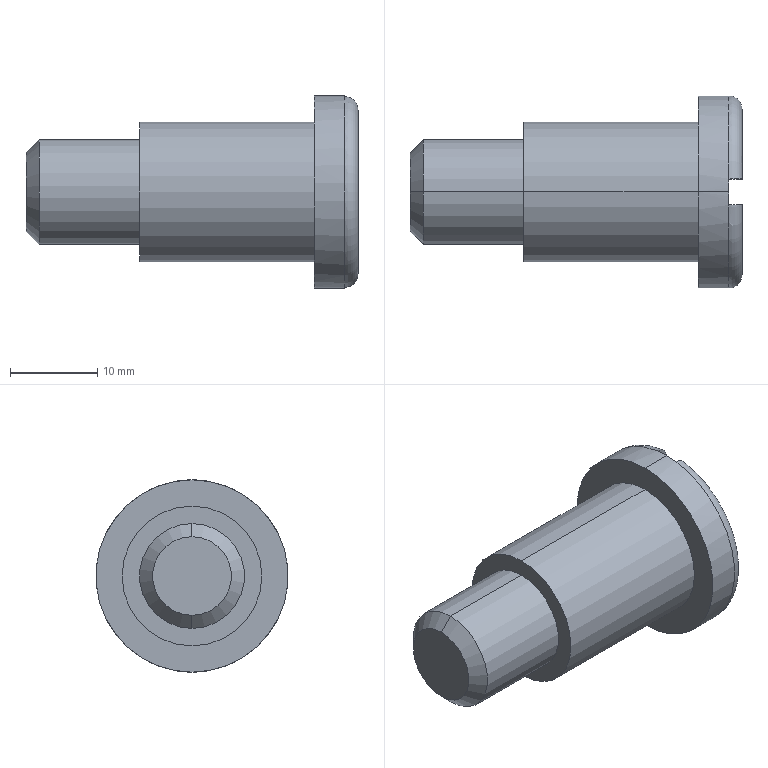Part | SolidWorks | features Chamfer 1, Cut 1, Fillet 1, Revolution 1 | 1 solid | 18 faces | box 38 x 22 x 22 mm | volume 7225 mm3 | plane 8 | cylinder 6 | cone 2 | torus 2 | commonest cylinder face diameters 12 x2 16 x2 22 x2
STEP:
#1=CARTESIAN_POINT('',(-19.,0.,4.5));
#2=VERTEX_POINT('',#1);
#3=CARTESIAN_POINT('',(-19.,0.,-4.5));
#4=VERTEX_POINT('',#3);
#5=CARTESIAN_POINT('',(-19.,0.,0.));
#6=DIRECTION('',(-1.,0.,0.));
#7=DIRECTION('',(0.,0.,-1.));
#8=AXIS2_PLACEMENT_3D('',#5,#6,#7);
#9=CIRCLE('',#8,4.5);
#10=EDGE_CURVE('',#2,#4,#9,.T.);
#11=ORIENTED_EDGE('',*,*,#10,.F.);
#12=CARTESIAN_POINT('',(-17.5,0.,6.));
#13=VERTEX_POINT('',#12);
#14=CARTESIAN_POINT('',(-19.,0.,4.5));
#15=DIRECTION('',(0.7071,0.,0.7071));
#16=VECTOR('',#15,1000.);
#17=LINE('',#14,#16);
#18=EDGE_CURVE('',#2,#13,#17,.T.);
#19=ORIENTED_EDGE('',*,*,#18,.T.);
#20=CARTESIAN_POINT('',(-17.5,0.,-6.));
#21=VERTEX_POINT('',#20);
#22=CARTESIAN_POINT('',(-17.5,0.,0.));
#23=DIRECTION('',(1.,0.,0.));
#24=DIRECTION('',(0.,0.,-1.));
#25=AXIS2_PLACEMENT_3D('',#22,#23,#24);
#26=CIRCLE('',#25,6.);
#27=EDGE_CURVE('',#21,#13,#26,.T.);
#28=ORIENTED_EDGE('',*,*,#27,.F.);
#29=CARTESIAN_POINT('',(-19.,0.,-4.5));
#30=DIRECTION('',(0.7071,0.,-0.7071));
#31=VECTOR('',#30,1000.);
#32=LINE('',#29,#31);
#33=EDGE_CURVE('',#4,#21,#32,.T.);
#34=ORIENTED_EDGE('',*,*,#33,.F.);
#35=EDGE_LOOP('',(#11,#19,#28,#34));
#36=FACE_OUTER_BOUND('',#35,.T.);
#37=CARTESIAN_POINT('',(-19.,0.,0.));
#38=DIRECTION('',(1.,0.,0.));
#39=DIRECTION('',(0.,0.,-1.));
#40=AXIS2_PLACEMENT_3D('',#37,#38,#39);
#41=CONICAL_SURFACE('',#40,4.5,0.7854);
#42=ADVANCED_FACE('',(#36),#41,.T.);
#43=CARTESIAN_POINT('',(-6.,0.,6.));
#44=VERTEX_POINT('',#43);
#45=CARTESIAN_POINT('',(-6.,0.,-6.));
#46=VERTEX_POINT('',#45);
#47=CARTESIAN_POINT('',(-6.,0.,0.));
#48=DIRECTION('',(-1.,0.,0.));
#49=DIRECTION('',(0.,0.,1.));
#50=AXIS2_PLACEMENT_3D('',#47,#48,#49);
#51=CIRCLE('',#50,6.);
#52=EDGE_CURVE('',#44,#46,#51,.T.);
#53=ORIENTED_EDGE('',*,*,#52,.T.);
#54=CARTESIAN_POINT('',(-19.,0.,-6.));
#55=DIRECTION('',(-1.,0.,0.));
#56=VECTOR('',#55,1000.);
#57=LINE('',#54,#56);
#58=EDGE_CURVE('',#46,#21,#57,.T.);
#59=ORIENTED_EDGE('',*,*,#58,.T.);
#60=ORIENTED_EDGE('',*,*,#27,.T.);
#61=CARTESIAN_POINT('',(-19.,0.,6.));
#62=DIRECTION('',(-1.,0.,0.));
#63=VECTOR('',#62,1000.);
#64=LINE('',#61,#63);
#65=EDGE_CURVE('',#44,#13,#64,.T.);
#66=ORIENTED_EDGE('',*,*,#65,.F.);
#67=EDGE_LOOP('',(#53,#59,#60,#66));
#68=FACE_OUTER_BOUND('',#67,.T.);
#69=CARTESIAN_POINT('',(-19.,0.,0.));
#70=DIRECTION('',(-1.,0.,0.));
#71=DIRECTION('',(0.,0.,1.));
#72=AXIS2_PLACEMENT_3D('',#69,#70,#71);
#73=CYLINDRICAL_SURFACE('',#72,6.);
#74=ADVANCED_FACE('',(#68),#73,.T.);
#75=CARTESIAN_POINT('',(14.,0.,8.));
#76=VERTEX_POINT('',#75);
#77=CARTESIAN_POINT('',(14.,0.,-8.));
#78=VERTEX_POINT('',#77);
#79=CARTESIAN_POINT('',(14.,0.,0.));
#80=DIRECTION('',(-1.,0.,0.));
#81=DIRECTION('',(0.,0.,1.));
#82=AXIS2_PLACEMENT_3D('',#79,#80,#81);
#83=CIRCLE('',#82,8.);
#84=EDGE_CURVE('',#76,#78,#83,.T.);
#85=ORIENTED_EDGE('',*,*,#84,.T.);
#86=CARTESIAN_POINT('',(-6.,0.,-8.));
#87=VERTEX_POINT('',#86);
#88=CARTESIAN_POINT('',(-19.,0.,-8.));
#89=DIRECTION('',(-1.,0.,0.));
#90=VECTOR('',#89,1000.);
#91=LINE('',#88,#90);
#92=EDGE_CURVE('',#78,#87,#91,.T.);
#93=ORIENTED_EDGE('',*,*,#92,.T.);
#94=CARTESIAN_POINT('',(-6.,0.,8.));
#95=VERTEX_POINT('',#94);
#96=CARTESIAN_POINT('',(-6.,0.,0.));
#97=DIRECTION('',(-1.,0.,0.));
#98=DIRECTION('',(0.,0.,1.));
#99=AXIS2_PLACEMENT_3D('',#96,#97,#98);
#100=CIRCLE('',#99,8.);
#101=EDGE_CURVE('',#95,#87,#100,.T.);
#102=ORIENTED_EDGE('',*,*,#101,.F.);
#103=CARTESIAN_POINT('',(-19.,0.,8.));
#104=DIRECTION('',(-1.,0.,0.));
#105=VECTOR('',#104,1000.);
#106=LINE('',#103,#105);
#107=EDGE_CURVE('',#76,#95,#106,.T.);
#108=ORIENTED_EDGE('',*,*,#107,.F.);
#109=EDGE_LOOP('',(#85,#93,#102,#108));
#110=FACE_OUTER_BOUND('',#109,.T.);
#111=CARTESIAN_POINT('',(-19.,0.,0.));
#112=DIRECTION('',(-1.,0.,0.));
#113=DIRECTION('',(0.,0.,1.));
#114=AXIS2_PLACEMENT_3D('',#111,#112,#113);
#115=CYLINDRICAL_SURFACE('',#114,8.);
#116=ADVANCED_FACE('',(#110),#115,.T.);
#117=CARTESIAN_POINT('',(17.5,0.,-11.));
#118=VERTEX_POINT('',#117);
#119=CARTESIAN_POINT('',(17.5,1.5,-10.897));
#120=VERTEX_POINT('',#119);
#121=CARTESIAN_POINT('',(17.5,0.,0.));
#122=DIRECTION('',(1.,0.,0.));
#123=DIRECTION('',(0.,0.,-1.));
#124=AXIS2_PLACEMENT_3D('',#121,#122,#123);
#125=CIRCLE('',#124,11.);
#126=EDGE_CURVE('',#118,#120,#125,.T.);
#127=ORIENTED_EDGE('',*,*,#126,.F.);
#128=CARTESIAN_POINT('',(14.,0.,-11.));
#129=VERTEX_POINT('',#128);
#130=CARTESIAN_POINT('',(-19.,0.,-11.));
#131=DIRECTION('',(-1.,0.,0.));
#132=VECTOR('',#131,1000.);
#133=LINE('',#130,#132);
#134=EDGE_CURVE('',#118,#129,#133,.T.);
#135=ORIENTED_EDGE('',*,*,#134,.T.);
#136=CARTESIAN_POINT('',(14.,0.,11.));
#137=VERTEX_POINT('',#136);
#138=CARTESIAN_POINT('',(14.,0.,0.));
#139=DIRECTION('',(-1.,0.,0.));
#140=DIRECTION('',(0.,0.,1.));
#141=AXIS2_PLACEMENT_3D('',#138,#139,#140);
#142=CIRCLE('',#141,11.);
#143=EDGE_CURVE('',#137,#129,#142,.T.);
#144=ORIENTED_EDGE('',*,*,#143,.F.);
#145=CARTESIAN_POINT('',(17.5,0.,11.));
#146=VERTEX_POINT('',#145);
#147=CARTESIAN_POINT('',(-19.,0.,11.));
#148=DIRECTION('',(-1.,0.,0.));
#149=VECTOR('',#148,1000.);
#150=LINE('',#147,#149);
#151=EDGE_CURVE('',#146,#137,#150,.T.);
#152=ORIENTED_EDGE('',*,*,#151,.F.);
#153=CARTESIAN_POINT('',(17.5,1.5,10.897));
#154=VERTEX_POINT('',#153);
#155=CARTESIAN_POINT('',(17.5,0.,0.));
#156=DIRECTION('',(1.,0.,0.));
#157=DIRECTION('',(0.,0.,-1.));
#158=AXIS2_PLACEMENT_3D('',#155,#156,#157);
#159=CIRCLE('',#158,11.);
#160=EDGE_CURVE('',#154,#146,#159,.T.);
#161=ORIENTED_EDGE('',*,*,#160,.F.);
#162=CARTESIAN_POINT('',(17.5,0.,0.));
#163=DIRECTION('',(-1.,0.,0.));
#164=DIRECTION('',(0.,0.,1.));
#165=AXIS2_PLACEMENT_3D('',#162,#163,#164);
#166=CIRCLE('',#165,11.);
#167=EDGE_CURVE('',#154,#120,#166,.T.);
#168=ORIENTED_EDGE('',*,*,#167,.T.);
#169=EDGE_LOOP('',(#127,#135,#144,#152,#161,#168));
#170=FACE_OUTER_BOUND('',#169,.T.);
#171=CARTESIAN_POINT('',(-19.,0.,0.));
#172=DIRECTION('',(-1.,0.,0.));
#173=DIRECTION('',(0.,0.,1.));
#174=AXIS2_PLACEMENT_3D('',#171,#172,#173);
#175=CYLINDRICAL_SURFACE('',#174,11.);
#176=ADVANCED_FACE('',(#170),#175,.T.);
#177=CARTESIAN_POINT('',(19.,1.5,-9.381));
#178=VERTEX_POINT('',#177);
#179=CARTESIAN_POINT('',(19.,1.5,9.381));
#180=VERTEX_POINT('',#179);
#181=CARTESIAN_POINT('',(19.,1.5,12.286));
#182=DIRECTION('',(0.,0.,1.));
#183=VECTOR('',#182,1000.);
#184=LINE('',#181,#183);
#185=EDGE_CURVE('',#178,#180,#184,.T.);
#186=ORIENTED_EDGE('',*,*,#185,.F.);
#187=CARTESIAN_POINT('',(19.,0.,0.));
#188=DIRECTION('',(1.,0.,0.));
#189=DIRECTION('',(0.,0.,1.));
#190=AXIS2_PLACEMENT_3D('',#187,#188,#189);
#191=CIRCLE('',#190,9.5);
#192=EDGE_CURVE('',#178,#180,#191,.T.);
#193=ORIENTED_EDGE('',*,*,#192,.T.);
#194=EDGE_LOOP('',(#186,#193));
#195=FACE_OUTER_BOUND('',#194,.T.);
#196=CARTESIAN_POINT('',(19.,0.,-11.));
#197=DIRECTION('',(-1.,0.,0.));
#198=DIRECTION('',(0.,0.,1.));
#199=AXIS2_PLACEMENT_3D('',#196,#197,#198);
#200=PLANE('',#199);
#201=ADVANCED_FACE('',(#195),#200,.F.);
#202=CARTESIAN_POINT('',(19.,-1.5,9.381));
#203=VERTEX_POINT('',#202);
#204=CARTESIAN_POINT('',(19.,-1.5,-9.381));
#205=VERTEX_POINT('',#204);
#206=CARTESIAN_POINT('',(19.,-1.5,12.286));
#207=DIRECTION('',(0.,0.,-1.));
#208=VECTOR('',#207,1000.);
#209=LINE('',#206,#208);
#210=EDGE_CURVE('',#203,#205,#209,.T.);
#211=ORIENTED_EDGE('',*,*,#210,.F.);
#212=CARTESIAN_POINT('',(19.,0.,0.));
#213=DIRECTION('',(1.,0.,0.));
#214=DIRECTION('',(0.,0.,1.));
#215=AXIS2_PLACEMENT_3D('',#212,#213,#214);
#216=CIRCLE('',#215,9.5);
#217=EDGE_CURVE('',#203,#205,#216,.T.);
#218=ORIENTED_EDGE('',*,*,#217,.T.);
#219=EDGE_LOOP('',(#211,#218));
#220=FACE_OUTER_BOUND('',#219,.T.);
#221=CARTESIAN_POINT('',(19.,0.,-11.));
#222=DIRECTION('',(-1.,0.,0.));
#223=DIRECTION('',(0.,0.,1.));
#224=AXIS2_PLACEMENT_3D('',#221,#222,#223);
#225=PLANE('',#224);
#226=ADVANCED_FACE('',(#220),#225,.F.);
#227=ORIENTED_EDGE('',*,*,#134,.F.);
#228=CARTESIAN_POINT('',(17.5,-1.5,-10.897));
#229=VERTEX_POINT('',#228);
#230=CARTESIAN_POINT('',(17.5,0.,0.));
#231=DIRECTION('',(1.,0.,0.));
#232=DIRECTION('',(0.,0.,-1.));
#233=AXIS2_PLACEMENT_3D('',#230,#231,#232);
#234=CIRCLE('',#233,11.);
#235=EDGE_CURVE('',#229,#118,#234,.T.);
#236=ORIENTED_EDGE('',*,*,#235,.F.);
#237=CARTESIAN_POINT('',(17.5,-1.5,10.897));
#238=VERTEX_POINT('',#237);
#239=CARTESIAN_POINT('',(17.5,0.,0.));
#240=DIRECTION('',(-1.,0.,0.));
#241=DIRECTION('',(0.,0.,1.));
#242=AXIS2_PLACEMENT_3D('',#239,#240,#241);
#243=CIRCLE('',#242,11.);
#244=EDGE_CURVE('',#229,#238,#243,.T.);
#245=ORIENTED_EDGE('',*,*,#244,.T.);
#246=CARTESIAN_POINT('',(17.5,0.,0.));
#247=DIRECTION('',(1.,0.,0.));
#248=DIRECTION('',(0.,0.,-1.));
#249=AXIS2_PLACEMENT_3D('',#246,#247,#248);
#250=CIRCLE('',#249,11.);
#251=EDGE_CURVE('',#146,#238,#250,.T.);
#252=ORIENTED_EDGE('',*,*,#251,.F.);
#253=ORIENTED_EDGE('',*,*,#151,.T.);
#254=CARTESIAN_POINT('',(14.,0.,0.));
#255=DIRECTION('',(-1.,0.,0.));
#256=DIRECTION('',(0.,0.,1.));
#257=AXIS2_PLACEMENT_3D('',#254,#255,#256);
#258=CIRCLE('',#257,11.);
#259=EDGE_CURVE('',#129,#137,#258,.T.);
#260=ORIENTED_EDGE('',*,*,#259,.F.);
#261=EDGE_LOOP('',(#227,#236,#245,#252,#253,#260));
#262=FACE_OUTER_BOUND('',#261,.T.);
#263=CARTESIAN_POINT('',(-19.,0.,0.));
#264=DIRECTION('',(-1.,0.,0.));
#265=DIRECTION('',(0.,0.,1.));
#266=AXIS2_PLACEMENT_3D('',#263,#264,#265);
#267=CYLINDRICAL_SURFACE('',#266,11.);
#268=ADVANCED_FACE('',(#262),#267,.T.);
#269=ORIENTED_EDGE('',*,*,#84,.F.);
#270=CARTESIAN_POINT('',(14.,0.,0.));
#271=DIRECTION('',(-1.,0.,0.));
#272=DIRECTION('',(0.,0.,1.));
#273=AXIS2_PLACEMENT_3D('',#270,#271,#272);
#274=CIRCLE('',#273,8.);
#275=EDGE_CURVE('',#78,#76,#274,.T.);
#276=ORIENTED_EDGE('',*,*,#275,.F.);
#277=EDGE_LOOP('',(#269,#276));
#278=FACE_BOUND('',#277,.T.);
#279=ORIENTED_EDGE('',*,*,#143,.T.);
#280=ORIENTED_EDGE('',*,*,#259,.T.);
#281=EDGE_LOOP('',(#279,#280));
#282=FACE_OUTER_BOUND('',#281,.T.);
#283=CARTESIAN_POINT('',(14.,0.,-8.));
#284=DIRECTION('',(1.,0.,0.));
#285=DIRECTION('',(0.,0.,-1.));
#286=AXIS2_PLACEMENT_3D('',#283,#284,#285);
#287=PLANE('',#286);
#288=ADVANCED_FACE('',(#278,#282),#287,.F.);
#289=ORIENTED_EDGE('',*,*,#92,.F.);
#290=ORIENTED_EDGE('',*,*,#275,.T.);
#291=ORIENTED_EDGE('',*,*,#107,.T.);
#292=CARTESIAN_POINT('',(-6.,0.,0.));
#293=DIRECTION('',(-1.,0.,0.));
#294=DIRECTION('',(0.,0.,1.));
#295=AXIS2_PLACEMENT_3D('',#292,#293,#294);
#296=CIRCLE('',#295,8.);
#297=EDGE_CURVE('',#87,#95,#296,.T.);
#298=ORIENTED_EDGE('',*,*,#297,.F.);
#299=EDGE_LOOP('',(#289,#290,#291,#298));
#300=FACE_OUTER_BOUND('',#299,.T.);
#301=CARTESIAN_POINT('',(-19.,0.,0.));
#302=DIRECTION('',(-1.,0.,0.));
#303=DIRECTION('',(0.,0.,1.));
#304=AXIS2_PLACEMENT_3D('',#301,#302,#303);
#305=CYLINDRICAL_SURFACE('',#304,8.);
#306=ADVANCED_FACE('',(#300),#305,.T.);
#307=ORIENTED_EDGE('',*,*,#52,.F.);
#308=CARTESIAN_POINT('',(-6.,0.,0.));
#309=DIRECTION('',(-1.,0.,0.));
#310=DIRECTION('',(0.,0.,1.));
#311=AXIS2_PLACEMENT_3D('',#308,#309,#310);
#312=CIRCLE('',#311,6.);
#313=EDGE_CURVE('',#46,#44,#312,.T.);
#314=ORIENTED_EDGE('',*,*,#313,.F.);
#315=EDGE_LOOP('',(#307,#314));
#316=FACE_BOUND('',#315,.T.);
#317=ORIENTED_EDGE('',*,*,#101,.T.);
#318=ORIENTED_EDGE('',*,*,#297,.T.);
#319=EDGE_LOOP('',(#317,#318));
#320=FACE_OUTER_BOUND('',#319,.T.);
#321=CARTESIAN_POINT('',(-6.,0.,-6.));
#322=DIRECTION('',(1.,0.,0.));
#323=DIRECTION('',(0.,0.,-1.));
#324=AXIS2_PLACEMENT_3D('',#321,#322,#323);
#325=PLANE('',#324);
#326=ADVANCED_FACE('',(#316,#320),#325,.F.);
#327=ORIENTED_EDGE('',*,*,#58,.F.);
#328=ORIENTED_EDGE('',*,*,#313,.T.);
#329=ORIENTED_EDGE('',*,*,#65,.T.);
#330=CARTESIAN_POINT('',(-17.5,0.,0.));
#331=DIRECTION('',(1.,0.,0.));
#332=DIRECTION('',(0.,0.,-1.));
#333=AXIS2_PLACEMENT_3D('',#330,#331,#332);
#334=CIRCLE('',#333,6.);
#335=EDGE_CURVE('',#13,#21,#334,.T.);
#336=ORIENTED_EDGE('',*,*,#335,.T.);
#337=EDGE_LOOP('',(#327,#328,#329,#336));
#338=FACE_OUTER_BOUND('',#337,.T.);
#339=CARTESIAN_POINT('',(-19.,0.,0.));
#340=DIRECTION('',(-1.,0.,0.));
#341=DIRECTION('',(0.,0.,1.));
#342=AXIS2_PLACEMENT_3D('',#339,#340,#341);
#343=CYLINDRICAL_SURFACE('',#342,6.);
#344=ADVANCED_FACE('',(#338),#343,.T.);
#345=CARTESIAN_POINT('',(-19.,0.,0.));
#346=DIRECTION('',(-1.,0.,0.));
#347=DIRECTION('',(0.,0.,-1.));
#348=AXIS2_PLACEMENT_3D('',#345,#346,#347);
#349=CIRCLE('',#348,4.5);
#350=EDGE_CURVE('',#4,#2,#349,.T.);
#351=ORIENTED_EDGE('',*,*,#350,.T.);
#352=ORIENTED_EDGE('',*,*,#10,.T.);
#353=EDGE_LOOP('',(#351,#352));
#354=FACE_OUTER_BOUND('',#353,.T.);
#355=CARTESIAN_POINT('',(-19.,0.,0.));
#356=DIRECTION('',(1.,0.,0.));
#357=DIRECTION('',(0.,0.,-1.));
#358=AXIS2_PLACEMENT_3D('',#355,#356,#357);
#359=PLANE('',#358);
#360=ADVANCED_FACE('',(#354),#359,.F.);
#361=CARTESIAN_POINT('',(17.5,1.5,12.286));
#362=DIRECTION('',(0.,0.,1.));
#363=VECTOR('',#362,1000.);
#364=LINE('',#361,#363);
#365=EDGE_CURVE('',#120,#154,#364,.T.);
#366=ORIENTED_EDGE('',*,*,#365,.F.);
#367=CARTESIAN_POINT('',(17.5,1.5,-10.897));
#368=CARTESIAN_POINT('',(17.6,1.5,-10.897));
#369=CARTESIAN_POINT('',(17.698,1.5,-10.887));
#370=CARTESIAN_POINT('',(17.89,1.5,-10.849));
#371=CARTESIAN_POINT('',(17.986,1.5,-10.819));
#372=CARTESIAN_POINT('',(18.168,1.5,-10.743));
#373=CARTESIAN_POINT('',(18.254,1.5,-10.696));
#374=CARTESIAN_POINT('',(18.417,1.5,-10.585));
#375=CARTESIAN_POINT('',(18.494,1.5,-10.521));
#376=CARTESIAN_POINT('',(18.701,1.5,-10.311));
#377=CARTESIAN_POINT('',(18.812,1.5,-10.142));
#378=CARTESIAN_POINT('',(18.961,1.5,-9.778));
#379=CARTESIAN_POINT('',(19.,1.5,-9.58));
#380=CARTESIAN_POINT('',(19.,1.5,-9.381));
#381=B_SPLINE_CURVE_WITH_KNOTS('',3,(#367,#368,#369,#370,#371,#372,#373,#374,#375,#376,#377,#378,#379,#380),.UNSPECIFIED.,.F.,.F.,(4,2,2,2,2,2,4),(0.,0.0002945,0.0005891,0.0008836,0.001178,0.001767,0.002356),.UNSPECIFIED.);
#382=EDGE_CURVE('',#120,#178,#381,.T.);
#383=ORIENTED_EDGE('',*,*,#382,.T.);
#384=ORIENTED_EDGE('',*,*,#185,.T.);
#385=CARTESIAN_POINT('',(19.,1.5,9.381));
#386=CARTESIAN_POINT('',(19.,1.5,9.48));
#387=CARTESIAN_POINT('',(18.99,1.5,9.578));
#388=CARTESIAN_POINT('',(18.953,1.5,9.771));
#389=CARTESIAN_POINT('',(18.924,1.5,9.867));
#390=CARTESIAN_POINT('',(18.85,1.5,10.05));
#391=CARTESIAN_POINT('',(18.804,1.5,10.137));
#392=CARTESIAN_POINT('',(18.696,1.5,10.302));
#393=CARTESIAN_POINT('',(18.633,1.5,10.38));
#394=CARTESIAN_POINT('',(18.426,1.5,10.59));
#395=CARTESIAN_POINT('',(18.259,1.5,10.704));
#396=CARTESIAN_POINT('',(17.897,1.5,10.857));
#397=CARTESIAN_POINT('',(17.699,1.5,10.897));
#398=CARTESIAN_POINT('',(17.5,1.5,10.897));
#399=B_SPLINE_CURVE_WITH_KNOTS('',3,(#385,#386,#387,#388,#389,#390,#391,#392,#393,#394,#395,#396,#397,#398),.UNSPECIFIED.,.F.,.F.,(4,2,2,2,2,2,4),(0.,0.0002945,0.0005891,0.0008836,0.001178,0.001767,0.002356),.UNSPECIFIED.);
#400=EDGE_CURVE('',#180,#154,#399,.T.);
#401=ORIENTED_EDGE('',*,*,#400,.T.);
#402=EDGE_LOOP('',(#366,#383,#384,#401));
#403=FACE_OUTER_BOUND('',#402,.T.);
#404=CARTESIAN_POINT('',(17.5,1.5,12.286));
#405=DIRECTION('',(0.,1.,0.));
#406=DIRECTION('',(0.,0.,1.));
#407=AXIS2_PLACEMENT_3D('',#404,#405,#406);
#408=PLANE('',#407);
#409=ADVANCED_FACE('',(#403),#408,.F.);
#410=CARTESIAN_POINT('',(17.5,-1.5,12.286));
#411=DIRECTION('',(0.,0.,-1.));
#412=VECTOR('',#411,1000.);
#413=LINE('',#410,#412);
#414=EDGE_CURVE('',#238,#229,#413,.T.);
#415=ORIENTED_EDGE('',*,*,#414,.F.);
#416=CARTESIAN_POINT('',(17.5,-1.5,10.897));
#417=CARTESIAN_POINT('',(17.6,-1.5,10.897));
#418=CARTESIAN_POINT('',(17.698,-1.5,10.887));
#419=CARTESIAN_POINT('',(17.89,-1.5,10.849));
#420=CARTESIAN_POINT('',(17.986,-1.5,10.819));
#421=CARTESIAN_POINT('',(18.168,-1.5,10.743));
#422=CARTESIAN_POINT('',(18.254,-1.5,10.696));
#423=CARTESIAN_POINT('',(18.417,-1.5,10.585));
#424=CARTESIAN_POINT('',(18.494,-1.5,10.521));
#425=CARTESIAN_POINT('',(18.701,-1.5,10.311));
#426=CARTESIAN_POINT('',(18.812,-1.5,10.142));
#427=CARTESIAN_POINT('',(18.961,-1.5,9.778));
#428=CARTESIAN_POINT('',(19.,-1.5,9.58));
#429=CARTESIAN_POINT('',(19.,-1.5,9.381));
#430=B_SPLINE_CURVE_WITH_KNOTS('',3,(#416,#417,#418,#419,#420,#421,#422,#423,#424,#425,#426,#427,#428,#429),.UNSPECIFIED.,.F.,.F.,(4,2,2,2,2,2,4),(0.,0.0002945,0.0005891,0.0008836,0.001178,0.001767,0.002356),.UNSPECIFIED.);
#431=EDGE_CURVE('',#238,#203,#430,.T.);
#432=ORIENTED_EDGE('',*,*,#431,.T.);
#433=ORIENTED_EDGE('',*,*,#210,.T.);
#434=CARTESIAN_POINT('',(19.,-1.5,-9.381));
#435=CARTESIAN_POINT('',(19.,-1.5,-9.48));
#436=CARTESIAN_POINT('',(18.99,-1.5,-9.578));
#437=CARTESIAN_POINT('',(18.953,-1.5,-9.771));
#438=CARTESIAN_POINT('',(18.924,-1.5,-9.867));
#439=CARTESIAN_POINT('',(18.85,-1.5,-10.05));
#440=CARTESIAN_POINT('',(18.804,-1.5,-10.137));
#441=CARTESIAN_POINT('',(18.696,-1.5,-10.302));
#442=CARTESIAN_POINT('',(18.633,-1.5,-10.38));
#443=CARTESIAN_POINT('',(18.426,-1.5,-10.59));
#444=CARTESIAN_POINT('',(18.259,-1.5,-10.704));
#445=CARTESIAN_POINT('',(17.897,-1.5,-10.857));
#446=CARTESIAN_POINT('',(17.699,-1.5,-10.897));
#447=CARTESIAN_POINT('',(17.5,-1.5,-10.897));
#448=B_SPLINE_CURVE_WITH_KNOTS('',3,(#434,#435,#436,#437,#438,#439,#440,#441,#442,#443,#444,#445,#446,#447),.UNSPECIFIED.,.F.,.F.,(4,2,2,2,2,2,4),(0.,0.0002945,0.0005891,0.0008836,0.001178,0.001767,0.002356),.UNSPECIFIED.);
#449=EDGE_CURVE('',#205,#229,#448,.T.);
#450=ORIENTED_EDGE('',*,*,#449,.T.);
#451=EDGE_LOOP('',(#415,#432,#433,#450));
#452=FACE_OUTER_BOUND('',#451,.T.);
#453=CARTESIAN_POINT('',(17.5,-1.5,12.286));
#454=DIRECTION('',(0.,-1.,0.));
#455=DIRECTION('',(0.,0.,-1.));
#456=AXIS2_PLACEMENT_3D('',#453,#454,#455);
#457=PLANE('',#456);
#458=ADVANCED_FACE('',(#452),#457,.F.);
#459=ORIENTED_EDGE('',*,*,#160,.T.);
#460=ORIENTED_EDGE('',*,*,#251,.T.);
#461=ORIENTED_EDGE('',*,*,#414,.T.);
#462=ORIENTED_EDGE('',*,*,#235,.T.);
#463=ORIENTED_EDGE('',*,*,#126,.T.);
#464=ORIENTED_EDGE('',*,*,#365,.T.);
#465=EDGE_LOOP('',(#459,#460,#461,#462,#463,#464));
#466=FACE_OUTER_BOUND('',#465,.T.);
#467=CARTESIAN_POINT('',(17.5,-1.5,12.286));
#468=DIRECTION('',(1.,0.,0.));
#469=DIRECTION('',(0.,0.,-1.));
#470=AXIS2_PLACEMENT_3D('',#467,#468,#469);
#471=PLANE('',#470);
#472=ADVANCED_FACE('',(#466),#471,.T.);
#473=ORIENTED_EDGE('',*,*,#449,.F.);
#474=ORIENTED_EDGE('',*,*,#217,.F.);
#475=ORIENTED_EDGE('',*,*,#431,.F.);
#476=ORIENTED_EDGE('',*,*,#244,.F.);
#477=EDGE_LOOP('',(#473,#474,#475,#476));
#478=FACE_OUTER_BOUND('',#477,.T.);
#479=CARTESIAN_POINT('',(17.5,0.,0.));
#480=DIRECTION('',(-1.,0.,0.));
#481=DIRECTION('',(0.,0.,1.));
#482=AXIS2_PLACEMENT_3D('',#479,#480,#481);
#483=TOROIDAL_SURFACE('',#482,9.5,1.5);
#484=ADVANCED_FACE('',(#478),#483,.T.);
#485=ORIENTED_EDGE('',*,*,#400,.F.);
#486=ORIENTED_EDGE('',*,*,#192,.F.);
#487=ORIENTED_EDGE('',*,*,#382,.F.);
#488=ORIENTED_EDGE('',*,*,#167,.F.);
#489=EDGE_LOOP('',(#485,#486,#487,#488));
#490=FACE_OUTER_BOUND('',#489,.T.);
#491=CARTESIAN_POINT('',(17.5,0.,0.));
#492=DIRECTION('',(-1.,0.,0.));
#493=DIRECTION('',(0.,0.,1.));
#494=AXIS2_PLACEMENT_3D('',#491,#492,#493);
#495=TOROIDAL_SURFACE('',#494,9.5,1.5);
#496=ADVANCED_FACE('',(#490),#495,.T.);
#497=ORIENTED_EDGE('',*,*,#18,.F.);
#498=ORIENTED_EDGE('',*,*,#350,.F.);
#499=ORIENTED_EDGE('',*,*,#33,.T.);
#500=ORIENTED_EDGE('',*,*,#335,.F.);
#501=EDGE_LOOP('',(#497,#498,#499,#500));
#502=FACE_OUTER_BOUND('',#501,.T.);
#503=CARTESIAN_POINT('',(-19.,0.,0.));
#504=DIRECTION('',(1.,0.,0.));
#505=DIRECTION('',(0.,0.,-1.));
#506=AXIS2_PLACEMENT_3D('',#503,#504,#505);
#507=CONICAL_SURFACE('',#506,4.5,0.7854);
#508=ADVANCED_FACE('',(#502),#507,.T.);
#509=CLOSED_SHELL('',(#42,#74,#116,#176,#201,#226,#268,#288,#306,#326,#344,#360,#409,#458,#472,#484,#496,#508));
#510=MANIFOLD_SOLID_BREP('',#509);
#511=CARTESIAN_POINT('',(0.,0.,0.));
#512=DIRECTION('',(0.,0.,1.));
#513=DIRECTION('',(1.,0.,0.));
#514=AXIS2_PLACEMENT_3D('',#511,#512,#513);
#515=(LENGTH_UNIT()NAMED_UNIT(*)SI_UNIT(.MILLI.,.METRE.));
#516=UNCERTAINTY_MEASURE_WITH_UNIT(LENGTH_MEASURE(0.00001),#515,'','');
#517=(NAMED_UNIT(*)PLANE_ANGLE_UNIT()SI_UNIT($,.RADIAN.));
#518=(NAMED_UNIT(*)SI_UNIT($,.STERADIAN.)SOLID_ANGLE_UNIT());
#519=(GEOMETRIC_REPRESENTATION_CONTEXT(3)GLOBAL_UNCERTAINTY_ASSIGNED_CONTEXT((#516))GLOBAL_UNIT_ASSIGNED_CONTEXT((#515,#517,#518))REPRESENTATION_CONTEXT('',''));
#520=ADVANCED_BREP_SHAPE_REPRESENTATION('',(#510,#514),#519);